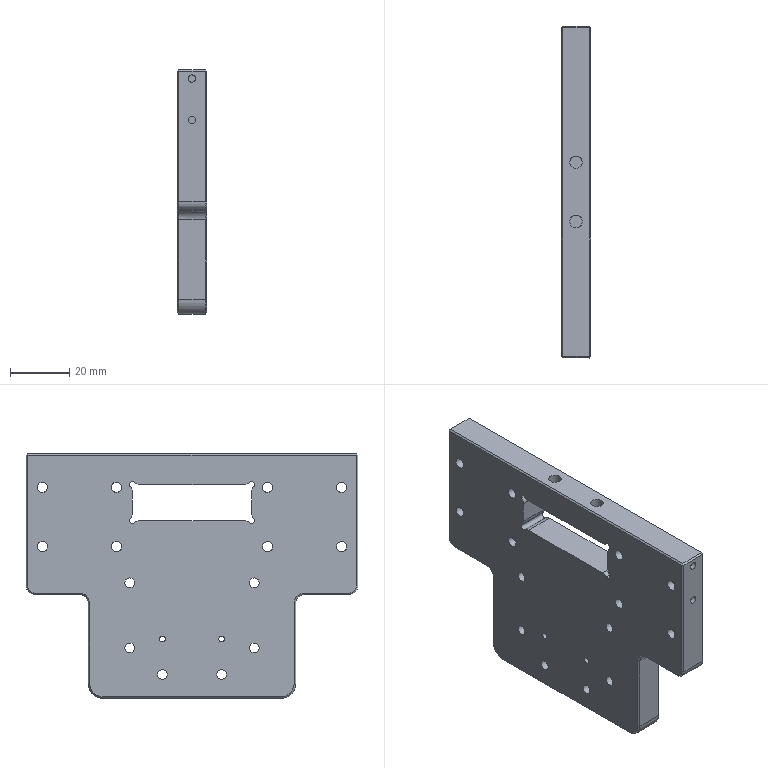CAM job | NX | 3+2 milling, drilling | part box 10 x 112 x 82.562 mm | stock box 12 x 117 x 87.562 mm
Tools:
number,name,description,diameter,corner_radius,flute_length,length,flutes
19,D2,平底铣刀-粗,2.0,0.0,50.0,75.0,2
4,D4,平底铣刀-粗,4.0,0.0,25.0,75.0,2
9,D10,平底铣刀-粗,10.0,0.0,35.0,75.0,2
20,D2-J,平底铣刀-精,2.0,0.0,50.0,75.0,2
11,D4-J,平底铣刀-精,4.0,0.0,50.0,75.0,2
7,D6-J,平底铣刀-精,6.0,0.0,25.0,75.0,2
1,D80R0.8FACEMILL,圆鼻刀-粗,80.0,0.8,50.0,75.0,2
1,D80R0.8FACEMILL-J,圆鼻刀-精,80.0,0.8,50.0,75.0,2
2,D6CHAMFERTOOL,倒角刀,6.0,0.0,3.0,25.0,2
21,M4X0.7,丝锥,3.3,0.0,35.0,50.0,2
17,ZT2,钻头,2.0,0.0,35.0,50.0,2
18,ZT3.5,钻头,3.5,0.0,35.0,50.0,2
13,DRILL3.3,Twist Drill 3.3 mm,3.3,0.0,35.0,35.008,2
Operations:
program,operation,operation_type,tool,method,geometry_group,spindle_rpm,surface_speed,feed_per_tooth,feed_cut,feed_plunge,cut_length_mm,path_length_mm,cut_time_min,machine_time_min
B,FLOORWALL_FACEMILL_ROUGH_COPY,VolumeBased25DMillingOperation,D80R0.8FACEMILL,LAYER_ROUGH-DEPTHK-STEPG,W-B,2800.0,703.696,0.5357,3000.0,100.0,1722.321,1839.079,0.5741,0.5858
B,FLOORWALL_FACEMILL_FINISH_COPY,VolumeBased25DMillingOperation,D80R0.8FACEMILL-J,SIDECUT_FINISH-DEPTHK-STEPG,W-B,4000.0,1005.28,0.125,1000.0,100.0,431.019,467.019,0.431,0.4346
B,DRILLCHAMFER_3,Operation,D6CHAMFERTOOL,METHOD,W-B,8000.0,150.796,0.0625,1000.0,0.0,8.6,80.424,0.0086,0.0158
B,DRILLCHAMFER_4,Operation,D6CHAMFERTOOL,METHOD,W-B,8000.0,150.796,0.0625,1000.0,0.0,40.4,324.142,0.0404,0.0688
B,DRILLCHAMFER_5,Operation,D6CHAMFERTOOL,METHOD,W-B,8000.0,150.796,0.0625,1000.0,0.0,31.2,211.083,0.0312,0.0492
B,C0.3_CLOSEDPROFILECHAMFER6X45L_COPY_1,PlanarMilling,D6CHAMFERTOOL,WALL_CHAMFER-DEPTH0-STEPG,W-B,7000.0,131.0,0.1071,1500.0,100.0,122.028,158.028,0.0814,0.085
B,C0.3_CLOSEDPROFILECHAMFER6X45L_COPY_2,PlanarMilling,D6CHAMFERTOOL,WALL_CHAMFER-DEPTH0-STEPG,W-B,7000.0,131.0,0.1071,1500.0,100.0,404.843,441.843,0.2699,0.2736
A,TOPFACE,FaceMilling,D80R0.8FACEMILL,SIDECUT_FINISH-DEPTHK-STEPG,W-A,4000.0,1005.31,0.125,1000.0,100.0,452.188,488.188,0.4522,0.4558
A,CAVITYMILL_ROUGH-MID_COPY,CavityMilling,D10,LAYER_ROUGH-DEPTHK-STEPG,W-A,8000.0,251.32,0.25,4000.0,100.0,23484.383,24003.821,5.871,5.949
A,WAISTSLOT_ROUGH_1,VolumeBased25DMillingOperation,D10,METHOD,W-A,6000.0,113.0,0.2083,2500.0,100.0,1537.541,1586.541,0.615,0.6199
A,SPOT-DEPTH0.8,Operation,D6CHAMFERTOOL,NONE,W-A,8000.0,150.796,0.0312,500.0,90.0,25.2,352.213,0.0504,0.0831
A,SPOT-DEPTH0.8_2,Operation,D6CHAMFERTOOL,NONE,W-A,8000.0,150.796,0.0312,500.0,90.0,3.6,68.225,0.0072,0.0137
A,THRUHOLE-PRECHOLE4.0_PREDRILL,Operation,ZT2,NONE,W-A,3000.0,36.757,0.0417,250.0,90.0,29.202,119.428,0.1168,0.1258
A,THRUHOLE-M4_TAPDRILL,Operation,DRILL3.3,NONE,W-A,3000.0,31.102,0.05,300.0,90.0,101.948,341.463,0.3398,0.3638
A,COUNTERBORE-DRILL_SEG0,Operation,ZT3.5,NONE,W-A,2800.0,30.788,0.0179,100.0,90.0,112.412,452.974,1.124,1.158
A,HOLEMILL_ROUGH_D2_1,CylinderMilling,D2,NONE,W-A,8000.0,50.266,0.0375,600.0,100.0,227.514,273.914,0.3792,0.3838
A,HOLEMILL_ROUGH_D2_2,CylinderMilling,D2,NONE,W-A,8000.0,50.266,0.0375,600.0,100.0,227.514,273.914,0.3792,0.3838
A,HOLEMILL_ROUGH_D4_1,CylinderMilling,D4,NONE,W-A,8000.0,100.531,0.075,1200.0,100.0,1200.422,1753.422,1,1.056
A,HOLEMILL_FINISH_D4_1,CylinderMilling,D4-J,FINISH_STEPDEPTH_OFF,W-A,8000.0,100.531,0.0312,500.0,100.0,170.919,723.919,0.3418,0.3971
A,CORNERCLEAN_D4,ZLevelMilling,D4-J,METHOD,W-A,6000.0,75.0,0.25,2500.0,80.0,1534.427,1627.709,0.614,0.6233
A,CORNERCLEAN_D2,ZLevelMilling,D2-J,METHOD,W-A,6000.0,37.699,0.125,1500.0,80.0,2276.234,2534.169,1.52,1.545
A,PROFILESIDE,ZLevelMilling,D6-J,METHOD,W-A,9000.0,84.823,0.1389,2500.0,80.0,553.151,728.847,0.2216,0.2392
A,DRILLCHAMFER_2,Operation,D6CHAMFERTOOL,METHOD,W-A,8000.0,150.796,0.0312,500.0,0.0,10.6,84.424,0.0212,0.0286
A,SELBODYONLY,SurfaceContour,D6CHAMFERTOOL,METHOD,W-A,8000.0,150.796,0.1875,3000.0,100.0,106.053,141.855,0.0354,0.0389
A,DRILLCHAMFER_1,Operation,D6CHAMFERTOOL,METHOD,W-A,8000.0,150.796,0.0312,500.0,0.0,31.2,211.083,0.0624,0.0804
A,MILLCHAMFER_1,PlanarMilling,D6CHAMFERTOOL,NONE,W-A,8000.0,150.796,0.0312,500.0,100.0,218.093,688.411,0.4362,0.4832
A,C0.3_CLOSEDPROFILECHAMFER6X45L_COPY,PlanarMilling,D6CHAMFERTOOL,WALL_CHAMFER-DEPTH0-STEPG,W-A,7000.0,131.0,0.1071,1500.0,100.0,404.843,441.843,0.2699,0.2736
A,THRUHOLE-TAP_M4,Operation,M4X0.7,METHOD,W-A,600.0,6.22,0.0006,0.7,90.0,84.0,305.566,120.0,120.022
A,WAISTSLOT_FINISH_1,VolumeBased25DMillingOperation,D4-J,METHOD,W-A,6000.0,75.398,0.0667,800.0,100.0,182.927,253.827,0.2287,0.2357
A,HOLEMILL_FINISH_D2_1,CylinderMilling,D2-J,FINISH_STEPDEPTH_OFF,W-A,8000.0,50.266,0.0125,200.0,100.0,33.701,80.001,0.1685,0.1731
A,HOLEMILL_FINISH_D2_2,CylinderMilling,D2-J,FINISH_STEPDEPTH_OFF,W-A,8000.0,50.266,0.0125,200.0,100.0,33.701,80.001,0.1685,0.1731
A,PROFILE_SEMIFINISH_2,VolumeBased25DMillingOperation,D6-J,METHOD,W-A,8000.0,251.327,0.0625,1000.0,100.0,402.84,462.04,0.4028,0.4088